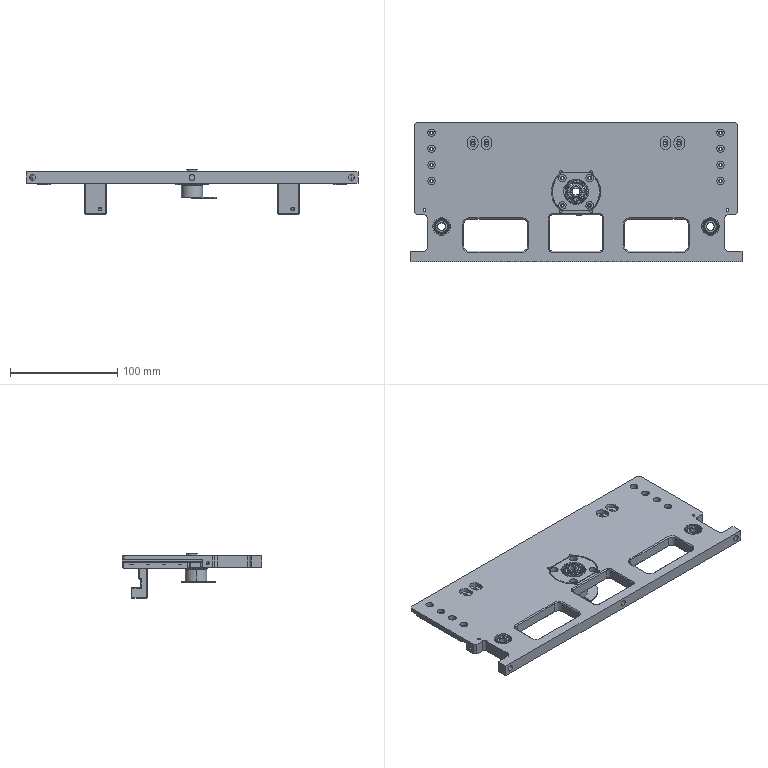Part | NX | features BREP 13 | 19 solids | 1425 faces | box 310 x 130.5 x 42 mm | volume 276547 mm3 | plane 510 | cylinder 456 | sphere 216 | cone 129 | torus 114 | commonest cylinder face diameters 2.5 x60 6 x44 10 x39 4.4 x32 7 x28 3.4 x24